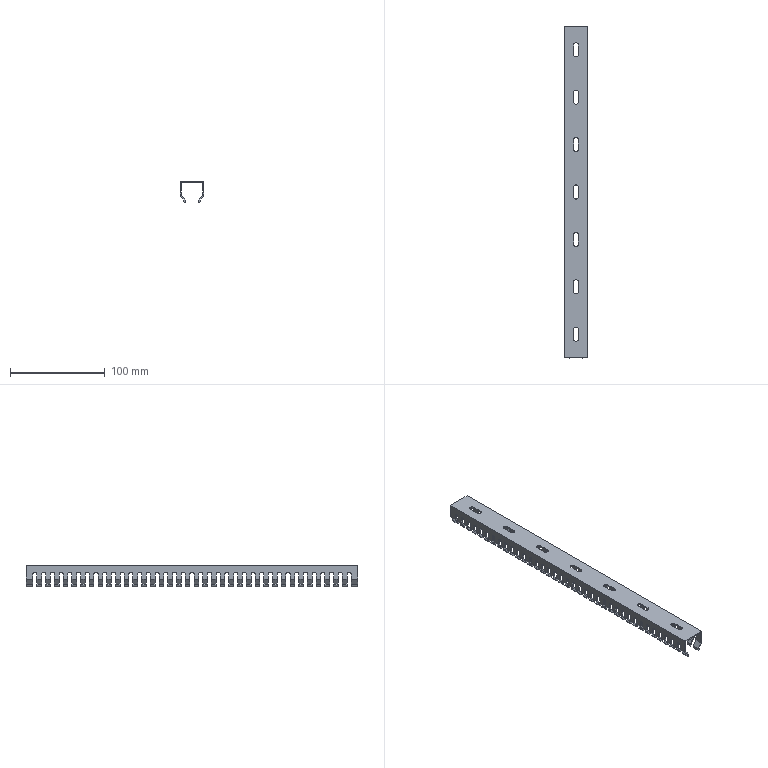Part | STEP file | Wire tray 25-23 | 1 solid | 938 faces | box 25.3 x 350 x 22.5 mm | volume 27781 mm3 | plane 624 | cylinder 314 | commonest cylinder face diameters 4 x148 0.6 x76 1 x76 5 x14